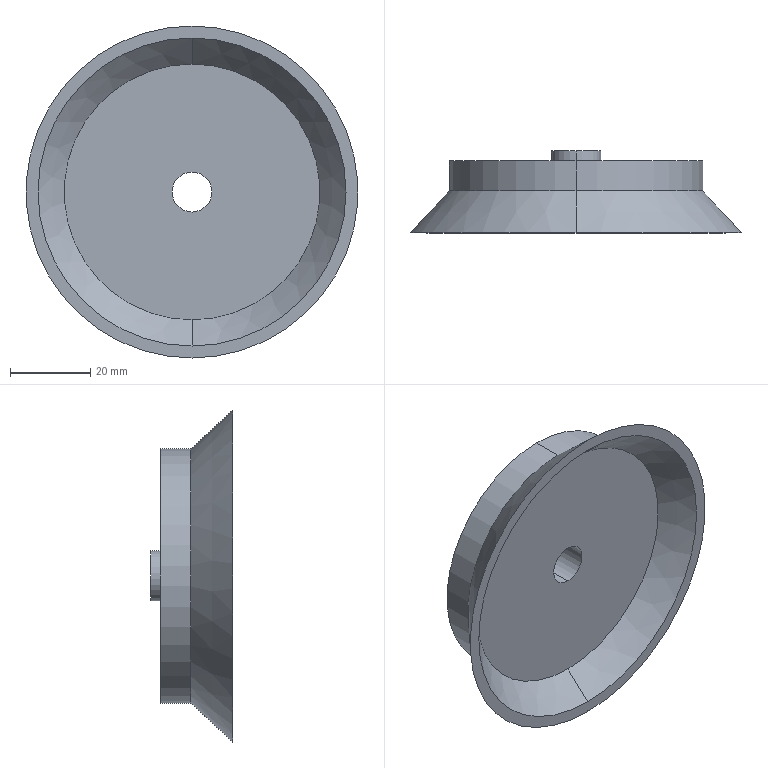Part | SolidWorks | features Revolution 1 | 1 solid | 14 faces | box 83 x 20.5 x 83 mm | volume 40041 mm3 | cylinder 6 | cone 4 | plane 4 | commonest cylinder face diameters 10 x2 12.5 x2 63.532 x2
STEP:
#1=CARTESIAN_POINT('',(0.,7.814,31.766));
#2=VERTEX_POINT('',#1);
#3=CARTESIAN_POINT('',(0.,7.814,-31.766));
#4=VERTEX_POINT('',#3);
#5=CARTESIAN_POINT('',(0.,7.814,0.));
#6=DIRECTION('',(0.,1.,0.));
#7=DIRECTION('',(0.,0.,1.));
#8=AXIS2_PLACEMENT_3D('',#5,#6,#7);
#9=CIRCLE('',#8,31.766);
#10=EDGE_CURVE('',#2,#4,#9,.T.);
#11=ORIENTED_EDGE('',*,*,#10,.T.);
#12=CARTESIAN_POINT('',(0.,15.314,-31.766));
#13=VERTEX_POINT('',#12);
#14=CARTESIAN_POINT('',(0.,20.559,-31.766));
#15=DIRECTION('',(0.,1.,0.));
#16=VECTOR('',#15,1000.);
#17=LINE('',#14,#16);
#18=EDGE_CURVE('',#4,#13,#17,.T.);
#19=ORIENTED_EDGE('',*,*,#18,.T.);
#20=CARTESIAN_POINT('',(0.,15.314,31.766));
#21=VERTEX_POINT('',#20);
#22=CARTESIAN_POINT('',(0.,15.314,0.));
#23=DIRECTION('',(0.,1.,0.));
#24=DIRECTION('',(0.,0.,1.));
#25=AXIS2_PLACEMENT_3D('',#22,#23,#24);
#26=CIRCLE('',#25,31.766);
#27=EDGE_CURVE('',#21,#13,#26,.T.);
#28=ORIENTED_EDGE('',*,*,#27,.F.);
#29=CARTESIAN_POINT('',(0.,20.559,31.766));
#30=DIRECTION('',(0.,1.,0.));
#31=VECTOR('',#30,1000.);
#32=LINE('',#29,#31);
#33=EDGE_CURVE('',#2,#21,#32,.T.);
#34=ORIENTED_EDGE('',*,*,#33,.F.);
#35=EDGE_LOOP('',(#11,#19,#28,#34));
#36=FACE_OUTER_BOUND('',#35,.T.);
#37=CARTESIAN_POINT('',(0.,20.559,0.));
#38=DIRECTION('',(0.,1.,0.));
#39=DIRECTION('',(0.,0.,1.));
#40=AXIS2_PLACEMENT_3D('',#37,#38,#39);
#41=CYLINDRICAL_SURFACE('',#40,31.766);
#42=ADVANCED_FACE('',(#36),#41,.T.);
#43=ORIENTED_EDGE('',*,*,#10,.F.);
#44=CARTESIAN_POINT('',(0.,-2.686,41.5));
#45=VERTEX_POINT('',#44);
#46=CARTESIAN_POINT('',(0.,7.814,31.766));
#47=DIRECTION('',(0.,-0.7333,0.6799));
#48=VECTOR('',#47,1000.);
#49=LINE('',#46,#48);
#50=EDGE_CURVE('',#2,#45,#49,.T.);
#51=ORIENTED_EDGE('',*,*,#50,.T.);
#52=CARTESIAN_POINT('',(0.,-2.686,-41.5));
#53=VERTEX_POINT('',#52);
#54=CARTESIAN_POINT('',(0.,-2.686,0.));
#55=DIRECTION('',(0.,1.,0.));
#56=DIRECTION('',(0.,0.,1.));
#57=AXIS2_PLACEMENT_3D('',#54,#55,#56);
#58=CIRCLE('',#57,41.5);
#59=EDGE_CURVE('',#45,#53,#58,.T.);
#60=ORIENTED_EDGE('',*,*,#59,.T.);
#61=CARTESIAN_POINT('',(0.,7.814,-31.766));
#62=DIRECTION('',(0.,-0.7333,-0.6799));
#63=VECTOR('',#62,1000.);
#64=LINE('',#61,#63);
#65=EDGE_CURVE('',#4,#53,#64,.T.);
#66=ORIENTED_EDGE('',*,*,#65,.F.);
#67=EDGE_LOOP('',(#43,#51,#60,#66));
#68=FACE_OUTER_BOUND('',#67,.T.);
#69=CARTESIAN_POINT('',(0.,7.814,0.));
#70=DIRECTION('',(0.,-1.,0.));
#71=DIRECTION('',(0.,0.,-1.));
#72=AXIS2_PLACEMENT_3D('',#69,#70,#71);
#73=CONICAL_SURFACE('',#72,31.766,0.7476);
#74=ADVANCED_FACE('',(#68),#73,.T.);
#75=CARTESIAN_POINT('',(0.,4.345,-31.981));
#76=VERTEX_POINT('',#75);
#77=CARTESIAN_POINT('',(0.,4.345,31.981));
#78=VERTEX_POINT('',#77);
#79=CARTESIAN_POINT('',(0.,4.345,0.));
#80=DIRECTION('',(0.,1.,0.));
#81=DIRECTION('',(0.,0.,1.));
#82=AXIS2_PLACEMENT_3D('',#79,#80,#81);
#83=CIRCLE('',#82,31.981);
#84=EDGE_CURVE('',#76,#78,#83,.T.);
#85=ORIENTED_EDGE('',*,*,#84,.T.);
#86=CARTESIAN_POINT('',(0.,-2.686,38.5));
#87=VERTEX_POINT('',#86);
#88=CARTESIAN_POINT('',(0.,-2.686,38.5));
#89=DIRECTION('',(0.,-0.7333,0.6799));
#90=VECTOR('',#89,1000.);
#91=LINE('',#88,#90);
#92=EDGE_CURVE('',#78,#87,#91,.T.);
#93=ORIENTED_EDGE('',*,*,#92,.T.);
#94=CARTESIAN_POINT('',(0.,-2.686,-38.5));
#95=VERTEX_POINT('',#94);
#96=CARTESIAN_POINT('',(0.,-2.686,0.));
#97=DIRECTION('',(0.,1.,0.));
#98=DIRECTION('',(0.,0.,1.));
#99=AXIS2_PLACEMENT_3D('',#96,#97,#98);
#100=CIRCLE('',#99,38.5);
#101=EDGE_CURVE('',#95,#87,#100,.T.);
#102=ORIENTED_EDGE('',*,*,#101,.F.);
#103=CARTESIAN_POINT('',(0.,-2.686,-38.5));
#104=DIRECTION('',(0.,-0.7333,-0.6799));
#105=VECTOR('',#104,1000.);
#106=LINE('',#103,#105);
#107=EDGE_CURVE('',#76,#95,#106,.T.);
#108=ORIENTED_EDGE('',*,*,#107,.F.);
#109=EDGE_LOOP('',(#85,#93,#102,#108));
#110=FACE_OUTER_BOUND('',#109,.T.);
#111=CARTESIAN_POINT('',(0.,-2.686,0.));
#112=DIRECTION('',(0.,-1.,0.));
#113=DIRECTION('',(0.,0.,-1.));
#114=AXIS2_PLACEMENT_3D('',#111,#112,#113);
#115=CONICAL_SURFACE('',#114,38.5,0.7476);
#116=ADVANCED_FACE('',(#110),#115,.F.);
#117=CARTESIAN_POINT('',(0.,4.345,-5.));
#118=VERTEX_POINT('',#117);
#119=CARTESIAN_POINT('',(0.,4.345,5.));
#120=VERTEX_POINT('',#119);
#121=CARTESIAN_POINT('',(0.,4.345,0.));
#122=DIRECTION('',(0.,1.,0.));
#123=DIRECTION('',(0.,0.,1.));
#124=AXIS2_PLACEMENT_3D('',#121,#122,#123);
#125=CIRCLE('',#124,5.);
#126=EDGE_CURVE('',#118,#120,#125,.T.);
#127=ORIENTED_EDGE('',*,*,#126,.F.);
#128=CARTESIAN_POINT('',(0.,17.814,-5.));
#129=VERTEX_POINT('',#128);
#130=CARTESIAN_POINT('',(0.,20.559,-5.));
#131=DIRECTION('',(0.,1.,0.));
#132=VECTOR('',#131,1000.);
#133=LINE('',#130,#132);
#134=EDGE_CURVE('',#118,#129,#133,.T.);
#135=ORIENTED_EDGE('',*,*,#134,.T.);
#136=CARTESIAN_POINT('',(0.,17.814,5.));
#137=VERTEX_POINT('',#136);
#138=CARTESIAN_POINT('',(0.,17.814,0.));
#139=DIRECTION('',(0.,1.,0.));
#140=DIRECTION('',(0.,0.,1.));
#141=AXIS2_PLACEMENT_3D('',#138,#139,#140);
#142=CIRCLE('',#141,5.);
#143=EDGE_CURVE('',#129,#137,#142,.T.);
#144=ORIENTED_EDGE('',*,*,#143,.T.);
#145=CARTESIAN_POINT('',(0.,20.559,5.));
#146=DIRECTION('',(0.,1.,0.));
#147=VECTOR('',#146,1000.);
#148=LINE('',#145,#147);
#149=EDGE_CURVE('',#120,#137,#148,.T.);
#150=ORIENTED_EDGE('',*,*,#149,.F.);
#151=EDGE_LOOP('',(#127,#135,#144,#150));
#152=FACE_OUTER_BOUND('',#151,.T.);
#153=CARTESIAN_POINT('',(0.,20.559,0.));
#154=DIRECTION('',(0.,1.,0.));
#155=DIRECTION('',(0.,0.,1.));
#156=AXIS2_PLACEMENT_3D('',#153,#154,#155);
#157=CYLINDRICAL_SURFACE('',#156,5.);
#158=ADVANCED_FACE('',(#152),#157,.F.);
#159=CARTESIAN_POINT('',(0.,15.314,6.25));
#160=VERTEX_POINT('',#159);
#161=CARTESIAN_POINT('',(0.,15.314,-6.25));
#162=VERTEX_POINT('',#161);
#163=CARTESIAN_POINT('',(0.,15.314,0.));
#164=DIRECTION('',(0.,1.,0.));
#165=DIRECTION('',(0.,0.,1.));
#166=AXIS2_PLACEMENT_3D('',#163,#164,#165);
#167=CIRCLE('',#166,6.25);
#168=EDGE_CURVE('',#160,#162,#167,.T.);
#169=ORIENTED_EDGE('',*,*,#168,.T.);
#170=CARTESIAN_POINT('',(0.,17.814,-6.25));
#171=VERTEX_POINT('',#170);
#172=CARTESIAN_POINT('',(0.,20.559,-6.25));
#173=DIRECTION('',(0.,1.,0.));
#174=VECTOR('',#173,1000.);
#175=LINE('',#172,#174);
#176=EDGE_CURVE('',#162,#171,#175,.T.);
#177=ORIENTED_EDGE('',*,*,#176,.T.);
#178=CARTESIAN_POINT('',(0.,17.814,6.25));
#179=VERTEX_POINT('',#178);
#180=CARTESIAN_POINT('',(0.,17.814,0.));
#181=DIRECTION('',(0.,1.,0.));
#182=DIRECTION('',(0.,0.,1.));
#183=AXIS2_PLACEMENT_3D('',#180,#181,#182);
#184=CIRCLE('',#183,6.25);
#185=EDGE_CURVE('',#179,#171,#184,.T.);
#186=ORIENTED_EDGE('',*,*,#185,.F.);
#187=CARTESIAN_POINT('',(0.,20.559,6.25));
#188=DIRECTION('',(0.,1.,0.));
#189=VECTOR('',#188,1000.);
#190=LINE('',#187,#189);
#191=EDGE_CURVE('',#160,#179,#190,.T.);
#192=ORIENTED_EDGE('',*,*,#191,.F.);
#193=EDGE_LOOP('',(#169,#177,#186,#192));
#194=FACE_OUTER_BOUND('',#193,.T.);
#195=CARTESIAN_POINT('',(0.,20.559,0.));
#196=DIRECTION('',(0.,1.,0.));
#197=DIRECTION('',(0.,0.,1.));
#198=AXIS2_PLACEMENT_3D('',#195,#196,#197);
#199=CYLINDRICAL_SURFACE('',#198,6.25);
#200=ADVANCED_FACE('',(#194),#199,.T.);
#201=ORIENTED_EDGE('',*,*,#176,.F.);
#202=CARTESIAN_POINT('',(0.,15.314,0.));
#203=DIRECTION('',(0.,1.,0.));
#204=DIRECTION('',(0.,0.,1.));
#205=AXIS2_PLACEMENT_3D('',#202,#203,#204);
#206=CIRCLE('',#205,6.25);
#207=EDGE_CURVE('',#162,#160,#206,.T.);
#208=ORIENTED_EDGE('',*,*,#207,.T.);
#209=ORIENTED_EDGE('',*,*,#191,.T.);
#210=CARTESIAN_POINT('',(0.,17.814,0.));
#211=DIRECTION('',(0.,1.,0.));
#212=DIRECTION('',(0.,0.,1.));
#213=AXIS2_PLACEMENT_3D('',#210,#211,#212);
#214=CIRCLE('',#213,6.25);
#215=EDGE_CURVE('',#171,#179,#214,.T.);
#216=ORIENTED_EDGE('',*,*,#215,.F.);
#217=EDGE_LOOP('',(#201,#208,#209,#216));
#218=FACE_OUTER_BOUND('',#217,.T.);
#219=CARTESIAN_POINT('',(0.,20.559,0.));
#220=DIRECTION('',(0.,1.,0.));
#221=DIRECTION('',(0.,0.,1.));
#222=AXIS2_PLACEMENT_3D('',#219,#220,#221);
#223=CYLINDRICAL_SURFACE('',#222,6.25);
#224=ADVANCED_FACE('',(#218),#223,.T.);
#225=ORIENTED_EDGE('',*,*,#185,.T.);
#226=ORIENTED_EDGE('',*,*,#215,.T.);
#227=EDGE_LOOP('',(#225,#226));
#228=FACE_OUTER_BOUND('',#227,.T.);
#229=CARTESIAN_POINT('',(0.,17.814,0.));
#230=DIRECTION('',(0.,1.,0.));
#231=DIRECTION('',(0.,0.,1.));
#232=AXIS2_PLACEMENT_3D('',#229,#230,#231);
#233=CIRCLE('',#232,5.);
#234=EDGE_CURVE('',#137,#129,#233,.T.);
#235=ORIENTED_EDGE('',*,*,#234,.F.);
#236=ORIENTED_EDGE('',*,*,#143,.F.);
#237=EDGE_LOOP('',(#235,#236));
#238=FACE_BOUND('',#237,.T.);
#239=CARTESIAN_POINT('',(-6.25,17.814,0.));
#240=DIRECTION('',(0.,1.,0.));
#241=DIRECTION('',(0.,0.,1.));
#242=AXIS2_PLACEMENT_3D('',#239,#240,#241);
#243=PLANE('',#242);
#244=ADVANCED_FACE('',(#228,#238),#243,.T.);
#245=ORIENTED_EDGE('',*,*,#134,.F.);
#246=CARTESIAN_POINT('',(0.,4.345,0.));
#247=DIRECTION('',(0.,1.,0.));
#248=DIRECTION('',(0.,0.,1.));
#249=AXIS2_PLACEMENT_3D('',#246,#247,#248);
#250=CIRCLE('',#249,5.);
#251=EDGE_CURVE('',#120,#118,#250,.T.);
#252=ORIENTED_EDGE('',*,*,#251,.F.);
#253=ORIENTED_EDGE('',*,*,#149,.T.);
#254=ORIENTED_EDGE('',*,*,#234,.T.);
#255=EDGE_LOOP('',(#245,#252,#253,#254));
#256=FACE_OUTER_BOUND('',#255,.T.);
#257=CARTESIAN_POINT('',(0.,20.559,0.));
#258=DIRECTION('',(0.,1.,0.));
#259=DIRECTION('',(0.,0.,1.));
#260=AXIS2_PLACEMENT_3D('',#257,#258,#259);
#261=CYLINDRICAL_SURFACE('',#260,5.);
#262=ADVANCED_FACE('',(#256),#261,.F.);
#263=ORIENTED_EDGE('',*,*,#251,.T.);
#264=ORIENTED_EDGE('',*,*,#126,.T.);
#265=EDGE_LOOP('',(#263,#264));
#266=FACE_BOUND('',#265,.T.);
#267=ORIENTED_EDGE('',*,*,#84,.F.);
#268=CARTESIAN_POINT('',(0.,4.345,0.));
#269=DIRECTION('',(0.,1.,0.));
#270=DIRECTION('',(0.,0.,1.));
#271=AXIS2_PLACEMENT_3D('',#268,#269,#270);
#272=CIRCLE('',#271,31.981);
#273=EDGE_CURVE('',#78,#76,#272,.T.);
#274=ORIENTED_EDGE('',*,*,#273,.F.);
#275=EDGE_LOOP('',(#267,#274));
#276=FACE_OUTER_BOUND('',#275,.T.);
#277=CARTESIAN_POINT('',(-31.981,4.345,0.));
#278=DIRECTION('',(0.,-1.,0.));
#279=DIRECTION('',(0.,0.,-1.));
#280=AXIS2_PLACEMENT_3D('',#277,#278,#279);
#281=PLANE('',#280);
#282=ADVANCED_FACE('',(#266,#276),#281,.T.);
#283=ORIENTED_EDGE('',*,*,#92,.F.);
#284=ORIENTED_EDGE('',*,*,#273,.T.);
#285=ORIENTED_EDGE('',*,*,#107,.T.);
#286=CARTESIAN_POINT('',(0.,-2.686,0.));
#287=DIRECTION('',(0.,1.,0.));
#288=DIRECTION('',(0.,0.,1.));
#289=AXIS2_PLACEMENT_3D('',#286,#287,#288);
#290=CIRCLE('',#289,38.5);
#291=EDGE_CURVE('',#87,#95,#290,.T.);
#292=ORIENTED_EDGE('',*,*,#291,.F.);
#293=EDGE_LOOP('',(#283,#284,#285,#292));
#294=FACE_OUTER_BOUND('',#293,.T.);
#295=CARTESIAN_POINT('',(0.,-2.686,0.));
#296=DIRECTION('',(0.,-1.,0.));
#297=DIRECTION('',(0.,0.,-1.));
#298=AXIS2_PLACEMENT_3D('',#295,#296,#297);
#299=CONICAL_SURFACE('',#298,38.5,0.7476);
#300=ADVANCED_FACE('',(#294),#299,.F.);
#301=ORIENTED_EDGE('',*,*,#101,.T.);
#302=ORIENTED_EDGE('',*,*,#291,.T.);
#303=EDGE_LOOP('',(#301,#302));
#304=FACE_BOUND('',#303,.T.);
#305=CARTESIAN_POINT('',(0.,-2.686,0.));
#306=DIRECTION('',(0.,1.,0.));
#307=DIRECTION('',(0.,0.,1.));
#308=AXIS2_PLACEMENT_3D('',#305,#306,#307);
#309=CIRCLE('',#308,41.5);
#310=EDGE_CURVE('',#53,#45,#309,.T.);
#311=ORIENTED_EDGE('',*,*,#310,.F.);
#312=ORIENTED_EDGE('',*,*,#59,.F.);
#313=EDGE_LOOP('',(#311,#312));
#314=FACE_OUTER_BOUND('',#313,.T.);
#315=CARTESIAN_POINT('',(-41.5,-2.686,0.));
#316=DIRECTION('',(0.,-1.,0.));
#317=DIRECTION('',(0.,0.,-1.));
#318=AXIS2_PLACEMENT_3D('',#315,#316,#317);
#319=PLANE('',#318);
#320=ADVANCED_FACE('',(#304,#314),#319,.T.);
#321=ORIENTED_EDGE('',*,*,#50,.F.);
#322=CARTESIAN_POINT('',(0.,7.814,0.));
#323=DIRECTION('',(0.,1.,0.));
#324=DIRECTION('',(0.,0.,1.));
#325=AXIS2_PLACEMENT_3D('',#322,#323,#324);
#326=CIRCLE('',#325,31.766);
#327=EDGE_CURVE('',#4,#2,#326,.T.);
#328=ORIENTED_EDGE('',*,*,#327,.F.);
#329=ORIENTED_EDGE('',*,*,#65,.T.);
#330=ORIENTED_EDGE('',*,*,#310,.T.);
#331=EDGE_LOOP('',(#321,#328,#329,#330));
#332=FACE_OUTER_BOUND('',#331,.T.);
#333=CARTESIAN_POINT('',(0.,7.814,0.));
#334=DIRECTION('',(0.,-1.,0.));
#335=DIRECTION('',(0.,0.,-1.));
#336=AXIS2_PLACEMENT_3D('',#333,#334,#335);
#337=CONICAL_SURFACE('',#336,31.766,0.7476);
#338=ADVANCED_FACE('',(#332),#337,.T.);
#339=ORIENTED_EDGE('',*,*,#18,.F.);
#340=ORIENTED_EDGE('',*,*,#327,.T.);
#341=ORIENTED_EDGE('',*,*,#33,.T.);
#342=CARTESIAN_POINT('',(0.,15.314,0.));
#343=DIRECTION('',(0.,1.,0.));
#344=DIRECTION('',(0.,0.,1.));
#345=AXIS2_PLACEMENT_3D('',#342,#343,#344);
#346=CIRCLE('',#345,31.766);
#347=EDGE_CURVE('',#13,#21,#346,.T.);
#348=ORIENTED_EDGE('',*,*,#347,.F.);
#349=EDGE_LOOP('',(#339,#340,#341,#348));
#350=FACE_OUTER_BOUND('',#349,.T.);
#351=CARTESIAN_POINT('',(0.,20.559,0.));
#352=DIRECTION('',(0.,1.,0.));
#353=DIRECTION('',(0.,0.,1.));
#354=AXIS2_PLACEMENT_3D('',#351,#352,#353);
#355=CYLINDRICAL_SURFACE('',#354,31.766);
#356=ADVANCED_FACE('',(#350),#355,.T.);
#357=ORIENTED_EDGE('',*,*,#27,.T.);
#358=ORIENTED_EDGE('',*,*,#347,.T.);
#359=EDGE_LOOP('',(#357,#358));
#360=FACE_OUTER_BOUND('',#359,.T.);
#361=ORIENTED_EDGE('',*,*,#168,.F.);
#362=ORIENTED_EDGE('',*,*,#207,.F.);
#363=EDGE_LOOP('',(#361,#362));
#364=FACE_BOUND('',#363,.T.);
#365=CARTESIAN_POINT('',(-6.25,15.314,0.));
#366=DIRECTION('',(0.,1.,0.));
#367=DIRECTION('',(0.,0.,1.));
#368=AXIS2_PLACEMENT_3D('',#365,#366,#367);
#369=PLANE('',#368);
#370=ADVANCED_FACE('',(#360,#364),#369,.T.);
#371=CLOSED_SHELL('',(#42,#74,#116,#158,#200,#224,#244,#262,#282,#300,#320,#338,#356,#370));
#372=MANIFOLD_SOLID_BREP('',#371);
#373=CARTESIAN_POINT('',(0.,0.,0.));
#374=DIRECTION('',(0.,0.,1.));
#375=DIRECTION('',(1.,0.,0.));
#376=AXIS2_PLACEMENT_3D('',#373,#374,#375);
#377=(LENGTH_UNIT()NAMED_UNIT(*)SI_UNIT(.MILLI.,.METRE.));
#378=UNCERTAINTY_MEASURE_WITH_UNIT(LENGTH_MEASURE(0.00001),#377,'','');
#379=(NAMED_UNIT(*)PLANE_ANGLE_UNIT()SI_UNIT($,.RADIAN.));
#380=(NAMED_UNIT(*)SI_UNIT($,.STERADIAN.)SOLID_ANGLE_UNIT());
#381=(GEOMETRIC_REPRESENTATION_CONTEXT(3)GLOBAL_UNCERTAINTY_ASSIGNED_CONTEXT((#378))GLOBAL_UNIT_ASSIGNED_CONTEXT((#377,#379,#380))REPRESENTATION_CONTEXT('',''));
#382=ADVANCED_BREP_SHAPE_REPRESENTATION('',(#372,#376),#381);